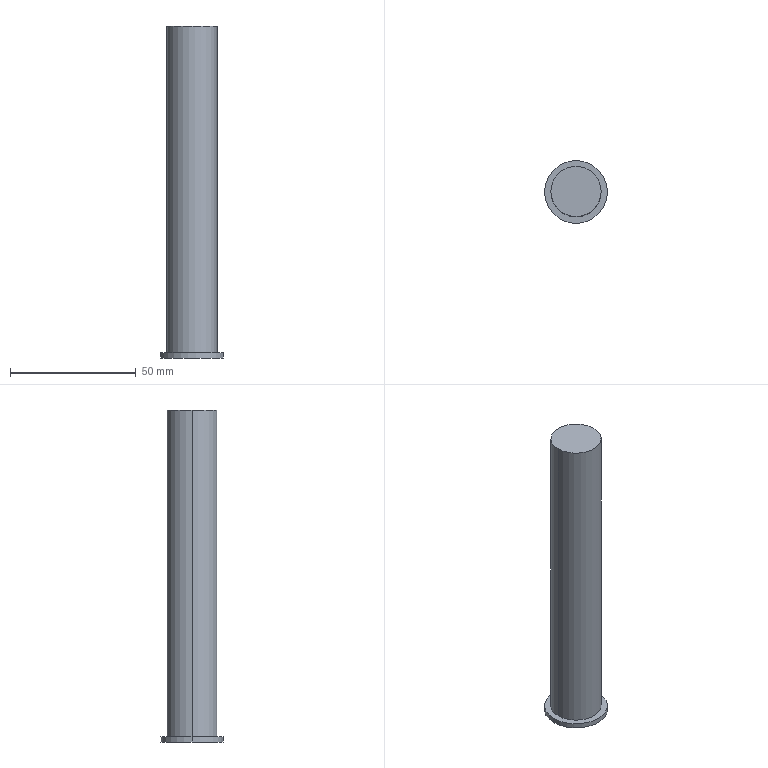Part | SolidWorks | features Extrusion 1, ICE 1 | 1 solid | 7 faces | box 25 x 25 x 132 mm | volume 41822 mm3 | cylinder 4 | plane 3 | commonest cylinder face diameters 20 x2 25 x2
STEP:
#1=CARTESIAN_POINT('',(10.,0.,132.));
#2=VERTEX_POINT('',#1);
#3=CARTESIAN_POINT('',(-10.,0.,132.));
#4=VERTEX_POINT('',#3);
#5=CARTESIAN_POINT('',(0.,0.,132.));
#6=DIRECTION('',(0.,0.,1.));
#7=DIRECTION('',(1.,0.,0.));
#8=AXIS2_PLACEMENT_3D('',#5,#6,#7);
#9=CIRCLE('',#8,10.);
#10=EDGE_CURVE('',#2,#4,#9,.T.);
#11=ORIENTED_EDGE('',*,*,#10,.F.);
#12=CARTESIAN_POINT('',(10.,0.,2.));
#13=VERTEX_POINT('',#12);
#14=CARTESIAN_POINT('',(10.,0.,132.));
#15=DIRECTION('',(0.,0.,-1.));
#16=VECTOR('',#15,1000.);
#17=LINE('',#14,#16);
#18=EDGE_CURVE('',#2,#13,#17,.T.);
#19=ORIENTED_EDGE('',*,*,#18,.T.);
#20=CARTESIAN_POINT('',(-10.,0.,2.));
#21=VERTEX_POINT('',#20);
#22=CARTESIAN_POINT('',(0.,0.,2.));
#23=DIRECTION('',(0.,0.,1.));
#24=DIRECTION('',(1.,0.,0.));
#25=AXIS2_PLACEMENT_3D('',#22,#23,#24);
#26=CIRCLE('',#25,10.);
#27=EDGE_CURVE('',#13,#21,#26,.T.);
#28=ORIENTED_EDGE('',*,*,#27,.T.);
#29=CARTESIAN_POINT('',(-10.,0.,132.));
#30=DIRECTION('',(0.,0.,-1.));
#31=VECTOR('',#30,1000.);
#32=LINE('',#29,#31);
#33=EDGE_CURVE('',#4,#21,#32,.T.);
#34=ORIENTED_EDGE('',*,*,#33,.F.);
#35=EDGE_LOOP('',(#11,#19,#28,#34));
#36=FACE_OUTER_BOUND('',#35,.T.);
#37=CARTESIAN_POINT('',(0.,0.,132.));
#38=DIRECTION('',(0.,0.,-1.));
#39=DIRECTION('',(-1.,0.,0.));
#40=AXIS2_PLACEMENT_3D('',#37,#38,#39);
#41=CYLINDRICAL_SURFACE('',#40,10.);
#42=ADVANCED_FACE('',(#36),#41,.T.);
#43=CARTESIAN_POINT('',(12.5,0.,2.));
#44=VERTEX_POINT('',#43);
#45=CARTESIAN_POINT('',(-12.5,0.,2.));
#46=VERTEX_POINT('',#45);
#47=CARTESIAN_POINT('',(0.,0.,2.));
#48=DIRECTION('',(0.,0.,1.));
#49=DIRECTION('',(1.,0.,0.));
#50=AXIS2_PLACEMENT_3D('',#47,#48,#49);
#51=CIRCLE('',#50,12.5);
#52=EDGE_CURVE('',#44,#46,#51,.T.);
#53=ORIENTED_EDGE('',*,*,#52,.F.);
#54=CARTESIAN_POINT('',(12.5,0.,0.));
#55=VERTEX_POINT('',#54);
#56=CARTESIAN_POINT('',(12.5,0.,2.));
#57=DIRECTION('',(0.,0.,-1.));
#58=VECTOR('',#57,1000.);
#59=LINE('',#56,#58);
#60=EDGE_CURVE('',#44,#55,#59,.T.);
#61=ORIENTED_EDGE('',*,*,#60,.T.);
#62=CARTESIAN_POINT('',(-12.5,0.,0.));
#63=VERTEX_POINT('',#62);
#64=CARTESIAN_POINT('',(0.,0.,0.));
#65=DIRECTION('',(0.,0.,1.));
#66=DIRECTION('',(1.,0.,0.));
#67=AXIS2_PLACEMENT_3D('',#64,#65,#66);
#68=CIRCLE('',#67,12.5);
#69=EDGE_CURVE('',#55,#63,#68,.T.);
#70=ORIENTED_EDGE('',*,*,#69,.T.);
#71=CARTESIAN_POINT('',(-12.5,0.,2.));
#72=DIRECTION('',(0.,0.,-1.));
#73=VECTOR('',#72,1000.);
#74=LINE('',#71,#73);
#75=EDGE_CURVE('',#46,#63,#74,.T.);
#76=ORIENTED_EDGE('',*,*,#75,.F.);
#77=EDGE_LOOP('',(#53,#61,#70,#76));
#78=FACE_OUTER_BOUND('',#77,.T.);
#79=CARTESIAN_POINT('',(0.,0.,2.));
#80=DIRECTION('',(0.,0.,-1.));
#81=DIRECTION('',(-1.,0.,0.));
#82=AXIS2_PLACEMENT_3D('',#79,#80,#81);
#83=CYLINDRICAL_SURFACE('',#82,12.5);
#84=ADVANCED_FACE('',(#78),#83,.T.);
#85=ORIENTED_EDGE('',*,*,#60,.F.);
#86=CARTESIAN_POINT('',(0.,0.,2.));
#87=DIRECTION('',(0.,0.,1.));
#88=DIRECTION('',(1.,0.,0.));
#89=AXIS2_PLACEMENT_3D('',#86,#87,#88);
#90=CIRCLE('',#89,12.5);
#91=EDGE_CURVE('',#46,#44,#90,.T.);
#92=ORIENTED_EDGE('',*,*,#91,.F.);
#93=ORIENTED_EDGE('',*,*,#75,.T.);
#94=CARTESIAN_POINT('',(0.,0.,0.));
#95=DIRECTION('',(0.,0.,1.));
#96=DIRECTION('',(1.,0.,0.));
#97=AXIS2_PLACEMENT_3D('',#94,#95,#96);
#98=CIRCLE('',#97,12.5);
#99=EDGE_CURVE('',#63,#55,#98,.T.);
#100=ORIENTED_EDGE('',*,*,#99,.T.);
#101=EDGE_LOOP('',(#85,#92,#93,#100));
#102=FACE_OUTER_BOUND('',#101,.T.);
#103=CARTESIAN_POINT('',(0.,0.,2.));
#104=DIRECTION('',(0.,0.,-1.));
#105=DIRECTION('',(-1.,0.,0.));
#106=AXIS2_PLACEMENT_3D('',#103,#104,#105);
#107=CYLINDRICAL_SURFACE('',#106,12.5);
#108=ADVANCED_FACE('',(#102),#107,.T.);
#109=CARTESIAN_POINT('',(0.,0.,2.));
#110=DIRECTION('',(0.,0.,1.));
#111=DIRECTION('',(1.,0.,0.));
#112=AXIS2_PLACEMENT_3D('',#109,#110,#111);
#113=CIRCLE('',#112,10.);
#114=EDGE_CURVE('',#21,#13,#113,.T.);
#115=ORIENTED_EDGE('',*,*,#114,.F.);
#116=ORIENTED_EDGE('',*,*,#27,.F.);
#117=EDGE_LOOP('',(#115,#116));
#118=FACE_BOUND('',#117,.T.);
#119=ORIENTED_EDGE('',*,*,#91,.T.);
#120=ORIENTED_EDGE('',*,*,#52,.T.);
#121=EDGE_LOOP('',(#119,#120));
#122=FACE_OUTER_BOUND('',#121,.T.);
#123=CARTESIAN_POINT('',(0.,0.,2.));
#124=DIRECTION('',(0.,0.,1.));
#125=DIRECTION('',(1.,0.,0.));
#126=AXIS2_PLACEMENT_3D('',#123,#124,#125);
#127=PLANE('',#126);
#128=ADVANCED_FACE('',(#118,#122),#127,.T.);
#129=ORIENTED_EDGE('',*,*,#99,.F.);
#130=ORIENTED_EDGE('',*,*,#69,.F.);
#131=EDGE_LOOP('',(#129,#130));
#132=FACE_OUTER_BOUND('',#131,.T.);
#133=CARTESIAN_POINT('',(0.,0.,0.));
#134=DIRECTION('',(0.,0.,1.));
#135=DIRECTION('',(1.,0.,0.));
#136=AXIS2_PLACEMENT_3D('',#133,#134,#135);
#137=PLANE('',#136);
#138=ADVANCED_FACE('',(#132),#137,.F.);
#139=ORIENTED_EDGE('',*,*,#18,.F.);
#140=CARTESIAN_POINT('',(0.,0.,132.));
#141=DIRECTION('',(0.,0.,1.));
#142=DIRECTION('',(1.,0.,0.));
#143=AXIS2_PLACEMENT_3D('',#140,#141,#142);
#144=CIRCLE('',#143,10.);
#145=EDGE_CURVE('',#4,#2,#144,.T.);
#146=ORIENTED_EDGE('',*,*,#145,.F.);
#147=ORIENTED_EDGE('',*,*,#33,.T.);
#148=ORIENTED_EDGE('',*,*,#114,.T.);
#149=EDGE_LOOP('',(#139,#146,#147,#148));
#150=FACE_OUTER_BOUND('',#149,.T.);
#151=CARTESIAN_POINT('',(0.,0.,132.));
#152=DIRECTION('',(0.,0.,-1.));
#153=DIRECTION('',(-1.,0.,0.));
#154=AXIS2_PLACEMENT_3D('',#151,#152,#153);
#155=CYLINDRICAL_SURFACE('',#154,10.);
#156=ADVANCED_FACE('',(#150),#155,.T.);
#157=ORIENTED_EDGE('',*,*,#145,.T.);
#158=ORIENTED_EDGE('',*,*,#10,.T.);
#159=EDGE_LOOP('',(#157,#158));
#160=FACE_OUTER_BOUND('',#159,.T.);
#161=CARTESIAN_POINT('',(0.,0.,132.));
#162=DIRECTION('',(0.,0.,1.));
#163=DIRECTION('',(1.,0.,0.));
#164=AXIS2_PLACEMENT_3D('',#161,#162,#163);
#165=PLANE('',#164);
#166=ADVANCED_FACE('',(#160),#165,.T.);
#167=CLOSED_SHELL('',(#42,#84,#108,#128,#138,#156,#166));
#168=MANIFOLD_SOLID_BREP('',#167);
#169=CARTESIAN_POINT('',(0.,0.,0.));
#170=DIRECTION('',(0.,0.,1.));
#171=DIRECTION('',(1.,0.,0.));
#172=AXIS2_PLACEMENT_3D('',#169,#170,#171);
#173=(LENGTH_UNIT()NAMED_UNIT(*)SI_UNIT(.MILLI.,.METRE.));
#174=UNCERTAINTY_MEASURE_WITH_UNIT(LENGTH_MEASURE(0.00001),#173,'','');
#175=(NAMED_UNIT(*)PLANE_ANGLE_UNIT()SI_UNIT($,.RADIAN.));
#176=(NAMED_UNIT(*)SI_UNIT($,.STERADIAN.)SOLID_ANGLE_UNIT());
#177=(GEOMETRIC_REPRESENTATION_CONTEXT(3)GLOBAL_UNCERTAINTY_ASSIGNED_CONTEXT((#174))GLOBAL_UNIT_ASSIGNED_CONTEXT((#173,#175,#176))REPRESENTATION_CONTEXT('',''));
#178=ADVANCED_BREP_SHAPE_REPRESENTATION('',(#168,#172),#177);